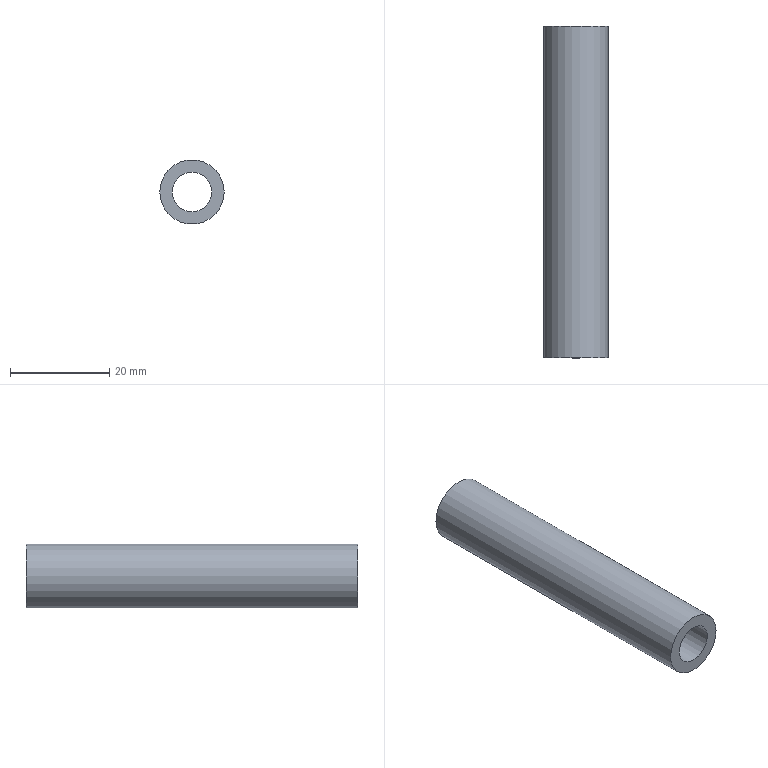Part | STEP file | 1-01.12 | 1 solid | 4 faces | box 13 x 67 x 13 mm | volume 5525 mm3 | plane 2 | cylinder 2 | commonest cylinder face diameters 8 x1 13 x1
STEP:
#1=CARTESIAN_POINT('',(0.,0.,0.));
#2=DIRECTION('',(0.,0.,1.));
#3=DIRECTION('',(1.,0.,0.));
#4=AXIS2_PLACEMENT_3D('',#1,#2,#3);
#5=CARTESIAN_POINT('',(6.5,33.5,0.));
#6=VERTEX_POINT('',#5);
#7=CARTESIAN_POINT('',(0.,33.5,0.));
#8=DIRECTION('',(0.,-1.,0.));
#9=DIRECTION('',(1.,0.,0.));
#10=AXIS2_PLACEMENT_3D('',#7,#8,#9);
#11=CIRCLE('',#10,6.5);
#12=CARTESIAN_POINT('',(-1.742,33.5,0.));
#13=DIRECTION('',(0.,-1.,0.));
#14=DIRECTION('',(1.,0.,0.));
#15=AXIS2_PLACEMENT_3D('',#12,#13,#14);
#16=PLANE('',#15);
#17=CARTESIAN_POINT('',(1.742,0.));
#18=DIRECTION('',(1.,0.));
#19=AXIS2_PLACEMENT_2D('',#17,#18);
#20=CIRCLE('',#19,6.5);
#21=(GEOMETRIC_REPRESENTATION_CONTEXT(2)PARAMETRIC_REPRESENTATION_CONTEXT()REPRESENTATION_CONTEXT('',''));
#22=DEFINITIONAL_REPRESENTATION('',(#20),#21);
#23=PCURVE('',#16,#22);
#24=CARTESIAN_POINT('',(0.,33.5,0.));
#25=DIRECTION('',(0.,-1.,0.));
#26=DIRECTION('',(1.,0.,0.));
#27=AXIS2_PLACEMENT_3D('',#24,#25,#26);
#28=CYLINDRICAL_SURFACE('',#27,6.5);
#29=CARTESIAN_POINT('',(0.,0.));
#30=DIRECTION('',(1.,0.));
#31=VECTOR('',#30,1.);
#32=LINE('',#29,#31);
#33=(GEOMETRIC_REPRESENTATION_CONTEXT(2)PARAMETRIC_REPRESENTATION_CONTEXT()REPRESENTATION_CONTEXT('',''));
#34=DEFINITIONAL_REPRESENTATION('',(#32),#33);
#35=PCURVE('',#28,#34);
#36=SURFACE_CURVE('',#11,(#23,#35),.PCURVE_S1.);
#37=EDGE_CURVE('',#6,#6,#36,.T.);
#38=ORIENTED_EDGE('',*,*,#37,.T.);
#39=EDGE_LOOP('',(#38));
#40=FACE_BOUND('',#39,.F.);
#41=CARTESIAN_POINT('',(4.,33.5,0.));
#42=VERTEX_POINT('',#41);
#43=CARTESIAN_POINT('',(0.,33.5,0.));
#44=DIRECTION('',(0.,1.,0.));
#45=DIRECTION('',(1.,0.,0.));
#46=AXIS2_PLACEMENT_3D('',#43,#44,#45);
#47=CIRCLE('',#46,4.);
#48=CARTESIAN_POINT('',(5.742,0.));
#49=CARTESIAN_POINT('',(5.742,-6.928));
#50=CARTESIAN_POINT('',(-0.2583,-3.464));
#51=CARTESIAN_POINT('',(-6.258,0.));
#52=CARTESIAN_POINT('',(-0.2583,3.464));
#53=CARTESIAN_POINT('',(5.742,6.928));
#54=CARTESIAN_POINT('',(5.742,0.));
#55=(BOUNDED_CURVE()B_SPLINE_CURVE(2,(#48,#49,#50,#51,#52,#53,#54),.UNSPECIFIED.,.T.,.F.)B_SPLINE_CURVE_WITH_KNOTS((1,2,2,2,2,1),(-2.094,0.,2.094,4.189,6.283,8.378),.UNSPECIFIED.)CURVE()GEOMETRIC_REPRESENTATION_ITEM()RATIONAL_B_SPLINE_CURVE((1.,0.5,1.,0.5,1.,0.5,1.))REPRESENTATION_ITEM(''));
#56=(GEOMETRIC_REPRESENTATION_CONTEXT(2)PARAMETRIC_REPRESENTATION_CONTEXT()REPRESENTATION_CONTEXT('',''));
#57=DEFINITIONAL_REPRESENTATION('',(#55),#56);
#58=PCURVE('',#16,#57);
#59=CARTESIAN_POINT('',(0.,33.5,0.));
#60=DIRECTION('',(0.,-1.,0.));
#61=DIRECTION('',(1.,0.,0.));
#62=AXIS2_PLACEMENT_3D('',#59,#60,#61);
#63=CYLINDRICAL_SURFACE('',#62,4.);
#64=CARTESIAN_POINT('',(6.283,0.));
#65=DIRECTION('',(-1.,0.));
#66=VECTOR('',#65,1.);
#67=LINE('',#64,#66);
#68=(GEOMETRIC_REPRESENTATION_CONTEXT(2)PARAMETRIC_REPRESENTATION_CONTEXT()REPRESENTATION_CONTEXT('',''));
#69=DEFINITIONAL_REPRESENTATION('',(#67),#68);
#70=PCURVE('',#63,#69);
#71=SURFACE_CURVE('',#47,(#58,#70),.PCURVE_S1.);
#72=EDGE_CURVE('',#42,#42,#71,.T.);
#73=ORIENTED_EDGE('',*,*,#72,.T.);
#74=EDGE_LOOP('',(#73));
#75=FACE_BOUND('',#74,.F.);
#76=ADVANCED_FACE('',(#40,#75),#16,.F.);
#77=CARTESIAN_POINT('',(6.5,-33.5,0.));
#78=VERTEX_POINT('',#77);
#79=CARTESIAN_POINT('',(0.,-33.5,0.));
#80=DIRECTION('',(0.,-1.,0.));
#81=DIRECTION('',(1.,0.,0.));
#82=AXIS2_PLACEMENT_3D('',#79,#80,#81);
#83=CIRCLE('',#82,6.5);
#84=CARTESIAN_POINT('',(-1.742,-33.5,0.));
#85=DIRECTION('',(0.,-1.,0.));
#86=DIRECTION('',(1.,0.,0.));
#87=AXIS2_PLACEMENT_3D('',#84,#85,#86);
#88=PLANE('',#87);
#89=CARTESIAN_POINT('',(1.742,0.));
#90=DIRECTION('',(1.,0.));
#91=AXIS2_PLACEMENT_2D('',#89,#90);
#92=CIRCLE('',#91,6.5);
#93=(GEOMETRIC_REPRESENTATION_CONTEXT(2)PARAMETRIC_REPRESENTATION_CONTEXT()REPRESENTATION_CONTEXT('',''));
#94=DEFINITIONAL_REPRESENTATION('',(#92),#93);
#95=PCURVE('',#88,#94);
#96=CARTESIAN_POINT('',(0.,67.));
#97=DIRECTION('',(1.,0.));
#98=VECTOR('',#97,1.);
#99=LINE('',#96,#98);
#100=(GEOMETRIC_REPRESENTATION_CONTEXT(2)PARAMETRIC_REPRESENTATION_CONTEXT()REPRESENTATION_CONTEXT('',''));
#101=DEFINITIONAL_REPRESENTATION('',(#99),#100);
#102=PCURVE('',#28,#101);
#103=SURFACE_CURVE('',#83,(#95,#102),.PCURVE_S1.);
#104=EDGE_CURVE('',#78,#78,#103,.T.);
#105=ORIENTED_EDGE('',*,*,#104,.T.);
#106=EDGE_LOOP('',(#105));
#107=FACE_BOUND('',#106,.T.);
#108=CARTESIAN_POINT('',(4.,-33.5,0.));
#109=VERTEX_POINT('',#108);
#110=CARTESIAN_POINT('',(0.,-33.5,0.));
#111=DIRECTION('',(0.,1.,0.));
#112=DIRECTION('',(1.,0.,0.));
#113=AXIS2_PLACEMENT_3D('',#110,#111,#112);
#114=CIRCLE('',#113,4.);
#115=CARTESIAN_POINT('',(5.742,0.));
#116=CARTESIAN_POINT('',(5.742,-6.928));
#117=CARTESIAN_POINT('',(-0.2583,-3.464));
#118=CARTESIAN_POINT('',(-6.258,0.));
#119=CARTESIAN_POINT('',(-0.2583,3.464));
#120=CARTESIAN_POINT('',(5.742,6.928));
#121=CARTESIAN_POINT('',(5.742,0.));
#122=(BOUNDED_CURVE()B_SPLINE_CURVE(2,(#115,#116,#117,#118,#119,#120,#121),.UNSPECIFIED.,.T.,.F.)B_SPLINE_CURVE_WITH_KNOTS((1,2,2,2,2,1),(-2.094,0.,2.094,4.189,6.283,8.378),.UNSPECIFIED.)CURVE()GEOMETRIC_REPRESENTATION_ITEM()RATIONAL_B_SPLINE_CURVE((1.,0.5,1.,0.5,1.,0.5,1.))REPRESENTATION_ITEM(''));
#123=(GEOMETRIC_REPRESENTATION_CONTEXT(2)PARAMETRIC_REPRESENTATION_CONTEXT()REPRESENTATION_CONTEXT('',''));
#124=DEFINITIONAL_REPRESENTATION('',(#122),#123);
#125=PCURVE('',#88,#124);
#126=CARTESIAN_POINT('',(6.283,67.));
#127=DIRECTION('',(-1.,0.));
#128=VECTOR('',#127,1.);
#129=LINE('',#126,#128);
#130=(GEOMETRIC_REPRESENTATION_CONTEXT(2)PARAMETRIC_REPRESENTATION_CONTEXT()REPRESENTATION_CONTEXT('',''));
#131=DEFINITIONAL_REPRESENTATION('',(#129),#130);
#132=PCURVE('',#63,#131);
#133=SURFACE_CURVE('',#114,(#125,#132),.PCURVE_S1.);
#134=EDGE_CURVE('',#109,#109,#133,.T.);
#135=ORIENTED_EDGE('',*,*,#134,.T.);
#136=EDGE_LOOP('',(#135));
#137=FACE_BOUND('',#136,.T.);
#138=ADVANCED_FACE('',(#107,#137),#88,.T.);
#139=ORIENTED_EDGE('',*,*,#37,.T.);
#140=CARTESIAN_POINT('',(6.5,33.5,0.));
#141=DIRECTION('',(0.,-1.,0.));
#142=VECTOR('',#141,1.);
#143=LINE('',#140,#142);
#144=CARTESIAN_POINT('',(6.283,0.));
#145=DIRECTION('',(0.,1.));
#146=VECTOR('',#145,1.);
#147=LINE('',#144,#146);
#148=(GEOMETRIC_REPRESENTATION_CONTEXT(2)PARAMETRIC_REPRESENTATION_CONTEXT()REPRESENTATION_CONTEXT('',''));
#149=DEFINITIONAL_REPRESENTATION('',(#147),#148);
#150=PCURVE('',#28,#149);
#151=CARTESIAN_POINT('',(0.,0.));
#152=DIRECTION('',(0.,1.));
#153=VECTOR('',#152,1.);
#154=LINE('',#151,#153);
#155=(GEOMETRIC_REPRESENTATION_CONTEXT(2)PARAMETRIC_REPRESENTATION_CONTEXT()REPRESENTATION_CONTEXT('',''));
#156=DEFINITIONAL_REPRESENTATION('',(#154),#155);
#157=PCURVE('',#28,#156);
#158=SEAM_CURVE('',#143,(#150,#157),.PCURVE_S1.);
#159=EDGE_CURVE('',#6,#78,#158,.T.);
#160=ORIENTED_EDGE('',*,*,#159,.T.);
#161=ORIENTED_EDGE('',*,*,#104,.F.);
#162=ORIENTED_EDGE('',*,*,#159,.F.);
#163=EDGE_LOOP('',(#139,#160,#161,#162));
#164=FACE_BOUND('',#163,.T.);
#165=ADVANCED_FACE('',(#164),#28,.T.);
#166=CARTESIAN_POINT('',(4.,33.5,0.));
#167=DIRECTION('',(0.,-1.,0.));
#168=VECTOR('',#167,1.);
#169=LINE('',#166,#168);
#170=CARTESIAN_POINT('',(6.283,0.));
#171=DIRECTION('',(0.,1.));
#172=VECTOR('',#171,1.);
#173=LINE('',#170,#172);
#174=(GEOMETRIC_REPRESENTATION_CONTEXT(2)PARAMETRIC_REPRESENTATION_CONTEXT()REPRESENTATION_CONTEXT('',''));
#175=DEFINITIONAL_REPRESENTATION('',(#173),#174);
#176=PCURVE('',#63,#175);
#177=CARTESIAN_POINT('',(0.,0.));
#178=DIRECTION('',(0.,1.));
#179=VECTOR('',#178,1.);
#180=LINE('',#177,#179);
#181=(GEOMETRIC_REPRESENTATION_CONTEXT(2)PARAMETRIC_REPRESENTATION_CONTEXT()REPRESENTATION_CONTEXT('',''));
#182=DEFINITIONAL_REPRESENTATION('',(#180),#181);
#183=PCURVE('',#63,#182);
#184=SEAM_CURVE('',#169,(#176,#183),.PCURVE_S1.);
#185=EDGE_CURVE('',#42,#109,#184,.T.);
#186=ORIENTED_EDGE('',*,*,#185,.T.);
#187=ORIENTED_EDGE('',*,*,#134,.T.);
#188=ORIENTED_EDGE('',*,*,#185,.F.);
#189=ORIENTED_EDGE('',*,*,#72,.F.);
#190=EDGE_LOOP('',(#186,#187,#188,#189));
#191=FACE_BOUND('',#190,.F.);
#192=ADVANCED_FACE('',(#191),#63,.F.);
#193=CLOSED_SHELL('',(#76,#138,#165,#192));
#194=MANIFOLD_SOLID_BREP('',#193);
#195=(LENGTH_UNIT()NAMED_UNIT(*)SI_UNIT(.MILLI.,.METRE.));
#196=UNCERTAINTY_MEASURE_WITH_UNIT(LENGTH_MEASURE(0.0000001),#195,'','');
#197=(NAMED_UNIT(*)PLANE_ANGLE_UNIT()SI_UNIT($,.RADIAN.));
#198=(NAMED_UNIT(*)SI_UNIT($,.STERADIAN.)SOLID_ANGLE_UNIT());
#199=(GEOMETRIC_REPRESENTATION_CONTEXT(3)GLOBAL_UNCERTAINTY_ASSIGNED_CONTEXT((#196))GLOBAL_UNIT_ASSIGNED_CONTEXT((#195,#197,#198))REPRESENTATION_CONTEXT('',''));
#200=ADVANCED_BREP_SHAPE_REPRESENTATION('',(#4,#194),#199);